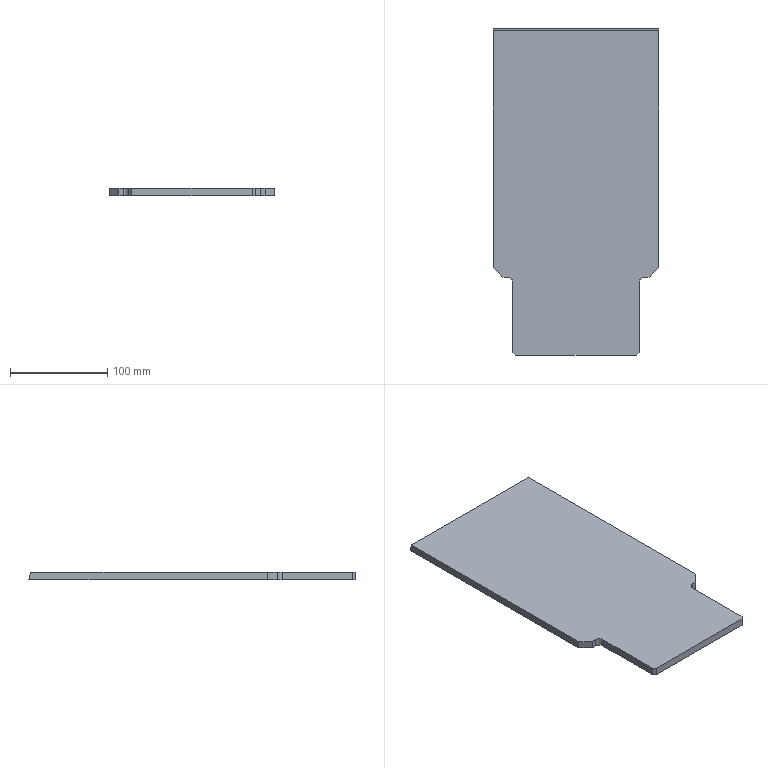Part | STEP file | 001-003-Feeding plate | 1 solid | 16 faces | box 170 x 335 x 8 mm | volume 427857 mm3 | plane 14 | cylinder 2 | commonest cylinder face diameters 10 x2
STEP:
#1=CARTESIAN_POINT('',(0.,0.,0.));
#2=DIRECTION('',(0.,0.,1.));
#3=DIRECTION('',(1.,0.,0.));
#4=AXIS2_PLACEMENT_3D('',#1,#2,#3);
#5=CARTESIAN_POINT('',(85.,-77.5,0.));
#6=VERTEX_POINT('',#5);
#7=CARTESIAN_POINT('',(85.,167.5,0.));
#8=VERTEX_POINT('',#7);
#9=CARTESIAN_POINT('',(85.,167.5,0.));
#10=DIRECTION('',(0.,1.,0.));
#11=VECTOR('',#10,1.);
#12=LINE('',#9,#11);
#13=CARTESIAN_POINT('',(85.,167.5,8.));
#14=DIRECTION('',(-1.,0.,0.));
#15=DIRECTION('',(0.,-1.,0.));
#16=AXIS2_PLACEMENT_3D('',#13,#14,#15);
#17=PLANE('',#16);
#18=CARTESIAN_POINT('',(0.,-8.));
#19=DIRECTION('',(-1.,0.));
#20=VECTOR('',#19,1.);
#21=LINE('',#18,#20);
#22=(GEOMETRIC_REPRESENTATION_CONTEXT(2)PARAMETRIC_REPRESENTATION_CONTEXT()REPRESENTATION_CONTEXT('',''));
#23=DEFINITIONAL_REPRESENTATION('',(#21),#22);
#24=PCURVE('',#17,#23);
#25=CARTESIAN_POINT('',(0.,0.,0.));
#26=DIRECTION('',(0.,0.,1.));
#27=DIRECTION('',(1.,0.,0.));
#28=AXIS2_PLACEMENT_3D('',#25,#26,#27);
#29=PLANE('',#28);
#30=CARTESIAN_POINT('',(85.,167.5));
#31=DIRECTION('',(0.,1.));
#32=VECTOR('',#31,1.);
#33=LINE('',#30,#32);
#34=(GEOMETRIC_REPRESENTATION_CONTEXT(2)PARAMETRIC_REPRESENTATION_CONTEXT()REPRESENTATION_CONTEXT('',''));
#35=DEFINITIONAL_REPRESENTATION('',(#33),#34);
#36=PCURVE('',#29,#35);
#37=SURFACE_CURVE('',#12,(#24,#36),.PCURVE_S1.);
#38=EDGE_CURVE('',#6,#8,#37,.T.);
#39=ORIENTED_EDGE('',*,*,#38,.T.);
#40=CARTESIAN_POINT('',(85.,165.505,8.));
#41=VERTEX_POINT('',#40);
#42=CARTESIAN_POINT('',(85.,167.5,0.));
#43=DIRECTION('',(0.,0.2419,-0.9703));
#44=VECTOR('',#43,1.);
#45=LINE('',#42,#44);
#46=CARTESIAN_POINT('',(0.,-8.));
#47=DIRECTION('',(-0.2419,-0.9703));
#48=VECTOR('',#47,1.);
#49=LINE('',#46,#48);
#50=(GEOMETRIC_REPRESENTATION_CONTEXT(2)PARAMETRIC_REPRESENTATION_CONTEXT()REPRESENTATION_CONTEXT('',''));
#51=DEFINITIONAL_REPRESENTATION('',(#49),#50);
#52=PCURVE('',#17,#51);
#53=CARTESIAN_POINT('',(-85.,167.5,0.));
#54=DIRECTION('',(0.,-0.9703,-0.2419));
#55=DIRECTION('',(0.,0.2419,-0.9703));
#56=AXIS2_PLACEMENT_3D('',#53,#54,#55);
#57=PLANE('',#56);
#58=CARTESIAN_POINT('',(0.,170.));
#59=DIRECTION('',(1.,0.));
#60=VECTOR('',#59,1.);
#61=LINE('',#58,#60);
#62=(GEOMETRIC_REPRESENTATION_CONTEXT(2)PARAMETRIC_REPRESENTATION_CONTEXT()REPRESENTATION_CONTEXT('',''));
#63=DEFINITIONAL_REPRESENTATION('',(#61),#62);
#64=PCURVE('',#57,#63);
#65=SURFACE_CURVE('',#45,(#52,#64),.PCURVE_S1.);
#66=EDGE_CURVE('',#41,#8,#65,.T.);
#67=ORIENTED_EDGE('',*,*,#66,.F.);
#68=CARTESIAN_POINT('',(85.,-77.5,8.));
#69=VERTEX_POINT('',#68);
#70=CARTESIAN_POINT('',(85.,167.5,8.));
#71=DIRECTION('',(0.,1.,0.));
#72=VECTOR('',#71,1.);
#73=LINE('',#70,#72);
#74=CARTESIAN_POINT('',(0.,0.));
#75=DIRECTION('',(-1.,0.));
#76=VECTOR('',#75,1.);
#77=LINE('',#74,#76);
#78=(GEOMETRIC_REPRESENTATION_CONTEXT(2)PARAMETRIC_REPRESENTATION_CONTEXT()REPRESENTATION_CONTEXT('',''));
#79=DEFINITIONAL_REPRESENTATION('',(#77),#78);
#80=PCURVE('',#17,#79);
#81=CARTESIAN_POINT('',(0.,0.,8.));
#82=DIRECTION('',(0.,0.,1.));
#83=DIRECTION('',(1.,0.,0.));
#84=AXIS2_PLACEMENT_3D('',#81,#82,#83);
#85=PLANE('',#84);
#86=CARTESIAN_POINT('',(85.,167.5));
#87=DIRECTION('',(0.,1.));
#88=VECTOR('',#87,1.);
#89=LINE('',#86,#88);
#90=(GEOMETRIC_REPRESENTATION_CONTEXT(2)PARAMETRIC_REPRESENTATION_CONTEXT()REPRESENTATION_CONTEXT('',''));
#91=DEFINITIONAL_REPRESENTATION('',(#89),#90);
#92=PCURVE('',#85,#91);
#93=SURFACE_CURVE('',#73,(#80,#92),.PCURVE_S1.);
#94=EDGE_CURVE('',#69,#41,#93,.T.);
#95=ORIENTED_EDGE('',*,*,#94,.F.);
#96=CARTESIAN_POINT('',(85.,-77.5,0.));
#97=DIRECTION('',(0.,0.,-1.));
#98=VECTOR('',#97,1.);
#99=LINE('',#96,#98);
#100=CARTESIAN_POINT('',(245.,-8.));
#101=DIRECTION('',(0.,-1.));
#102=VECTOR('',#101,1.);
#103=LINE('',#100,#102);
#104=(GEOMETRIC_REPRESENTATION_CONTEXT(2)PARAMETRIC_REPRESENTATION_CONTEXT()REPRESENTATION_CONTEXT('',''));
#105=DEFINITIONAL_REPRESENTATION('',(#103),#104);
#106=PCURVE('',#17,#105);
#107=CARTESIAN_POINT('',(85.,-77.5,8.));
#108=DIRECTION('',(0.7071,-0.7071,0.));
#109=DIRECTION('',(0.,0.,1.));
#110=AXIS2_PLACEMENT_3D('',#107,#108,#109);
#111=PLANE('',#110);
#112=CARTESIAN_POINT('',(-8.,0.));
#113=DIRECTION('',(-1.,0.));
#114=VECTOR('',#113,1.);
#115=LINE('',#112,#114);
#116=(GEOMETRIC_REPRESENTATION_CONTEXT(2)PARAMETRIC_REPRESENTATION_CONTEXT()REPRESENTATION_CONTEXT('',''));
#117=DEFINITIONAL_REPRESENTATION('',(#115),#116);
#118=PCURVE('',#111,#117);
#119=SURFACE_CURVE('',#99,(#106,#118),.PCURVE_S1.);
#120=EDGE_CURVE('',#69,#6,#119,.T.);
#121=ORIENTED_EDGE('',*,*,#120,.T.);
#122=EDGE_LOOP('',(#39,#67,#95,#121));
#123=FACE_BOUND('',#122,.T.);
#124=ADVANCED_FACE('',(#123),#17,.F.);
#125=CARTESIAN_POINT('',(-85.,165.505,8.));
#126=VERTEX_POINT('',#125);
#127=CARTESIAN_POINT('',(-85.,-77.5,8.));
#128=VERTEX_POINT('',#127);
#129=CARTESIAN_POINT('',(-85.,167.5,8.));
#130=DIRECTION('',(0.,-1.,0.));
#131=VECTOR('',#130,1.);
#132=LINE('',#129,#131);
#133=CARTESIAN_POINT('',(-85.,167.5,8.));
#134=DIRECTION('',(1.,0.,0.));
#135=DIRECTION('',(0.,1.,0.));
#136=AXIS2_PLACEMENT_3D('',#133,#134,#135);
#137=PLANE('',#136);
#138=CARTESIAN_POINT('',(0.,0.));
#139=DIRECTION('',(-1.,0.));
#140=VECTOR('',#139,1.);
#141=LINE('',#138,#140);
#142=(GEOMETRIC_REPRESENTATION_CONTEXT(2)PARAMETRIC_REPRESENTATION_CONTEXT()REPRESENTATION_CONTEXT('',''));
#143=DEFINITIONAL_REPRESENTATION('',(#141),#142);
#144=PCURVE('',#137,#143);
#145=CARTESIAN_POINT('',(-85.,167.5));
#146=DIRECTION('',(0.,-1.));
#147=VECTOR('',#146,1.);
#148=LINE('',#145,#147);
#149=(GEOMETRIC_REPRESENTATION_CONTEXT(2)PARAMETRIC_REPRESENTATION_CONTEXT()REPRESENTATION_CONTEXT('',''));
#150=DEFINITIONAL_REPRESENTATION('',(#148),#149);
#151=PCURVE('',#85,#150);
#152=SURFACE_CURVE('',#132,(#144,#151),.PCURVE_S1.);
#153=EDGE_CURVE('',#126,#128,#152,.T.);
#154=ORIENTED_EDGE('',*,*,#153,.F.);
#155=CARTESIAN_POINT('',(-85.,167.5,0.));
#156=VERTEX_POINT('',#155);
#157=CARTESIAN_POINT('',(-85.,167.5,0.));
#158=DIRECTION('',(0.,0.2419,-0.9703));
#159=VECTOR('',#158,1.);
#160=LINE('',#157,#159);
#161=CARTESIAN_POINT('',(0.,-8.));
#162=DIRECTION('',(0.2419,-0.9703));
#163=VECTOR('',#162,1.);
#164=LINE('',#161,#163);
#165=(GEOMETRIC_REPRESENTATION_CONTEXT(2)PARAMETRIC_REPRESENTATION_CONTEXT()REPRESENTATION_CONTEXT('',''));
#166=DEFINITIONAL_REPRESENTATION('',(#164),#165);
#167=PCURVE('',#137,#166);
#168=CARTESIAN_POINT('',(0.,0.));
#169=DIRECTION('',(1.,0.));
#170=VECTOR('',#169,1.);
#171=LINE('',#168,#170);
#172=(GEOMETRIC_REPRESENTATION_CONTEXT(2)PARAMETRIC_REPRESENTATION_CONTEXT()REPRESENTATION_CONTEXT('',''));
#173=DEFINITIONAL_REPRESENTATION('',(#171),#172);
#174=PCURVE('',#57,#173);
#175=SURFACE_CURVE('',#160,(#167,#174),.PCURVE_S1.);
#176=EDGE_CURVE('',#126,#156,#175,.T.);
#177=ORIENTED_EDGE('',*,*,#176,.T.);
#178=CARTESIAN_POINT('',(-85.,-77.5,0.));
#179=VERTEX_POINT('',#178);
#180=CARTESIAN_POINT('',(-85.,167.5,0.));
#181=DIRECTION('',(0.,-1.,0.));
#182=VECTOR('',#181,1.);
#183=LINE('',#180,#182);
#184=CARTESIAN_POINT('',(0.,-8.));
#185=DIRECTION('',(-1.,0.));
#186=VECTOR('',#185,1.);
#187=LINE('',#184,#186);
#188=(GEOMETRIC_REPRESENTATION_CONTEXT(2)PARAMETRIC_REPRESENTATION_CONTEXT()REPRESENTATION_CONTEXT('',''));
#189=DEFINITIONAL_REPRESENTATION('',(#187),#188);
#190=PCURVE('',#137,#189);
#191=CARTESIAN_POINT('',(-85.,167.5));
#192=DIRECTION('',(0.,-1.));
#193=VECTOR('',#192,1.);
#194=LINE('',#191,#193);
#195=(GEOMETRIC_REPRESENTATION_CONTEXT(2)PARAMETRIC_REPRESENTATION_CONTEXT()REPRESENTATION_CONTEXT('',''));
#196=DEFINITIONAL_REPRESENTATION('',(#194),#195);
#197=PCURVE('',#29,#196);
#198=SURFACE_CURVE('',#183,(#190,#197),.PCURVE_S1.);
#199=EDGE_CURVE('',#156,#179,#198,.T.);
#200=ORIENTED_EDGE('',*,*,#199,.T.);
#201=CARTESIAN_POINT('',(-85.,-77.5,8.));
#202=DIRECTION('',(0.,0.,1.));
#203=VECTOR('',#202,1.);
#204=LINE('',#201,#203);
#205=CARTESIAN_POINT('',(-245.,0.));
#206=DIRECTION('',(0.,1.));
#207=VECTOR('',#206,1.);
#208=LINE('',#205,#207);
#209=(GEOMETRIC_REPRESENTATION_CONTEXT(2)PARAMETRIC_REPRESENTATION_CONTEXT()REPRESENTATION_CONTEXT('',''));
#210=DEFINITIONAL_REPRESENTATION('',(#208),#209);
#211=PCURVE('',#137,#210);
#212=CARTESIAN_POINT('',(-75.,-87.5,8.));
#213=DIRECTION('',(-0.7071,-0.7071,0.));
#214=DIRECTION('',(0.,0.,1.));
#215=AXIS2_PLACEMENT_3D('',#212,#213,#214);
#216=PLANE('',#215);
#217=CARTESIAN_POINT('',(0.,14.142));
#218=DIRECTION('',(1.,0.));
#219=VECTOR('',#218,1.);
#220=LINE('',#217,#219);
#221=(GEOMETRIC_REPRESENTATION_CONTEXT(2)PARAMETRIC_REPRESENTATION_CONTEXT()REPRESENTATION_CONTEXT('',''));
#222=DEFINITIONAL_REPRESENTATION('',(#220),#221);
#223=PCURVE('',#216,#222);
#224=SURFACE_CURVE('',#204,(#211,#223),.PCURVE_S1.);
#225=EDGE_CURVE('',#179,#128,#224,.T.);
#226=ORIENTED_EDGE('',*,*,#225,.T.);
#227=EDGE_LOOP('',(#154,#177,#200,#226));
#228=FACE_BOUND('',#227,.T.);
#229=ADVANCED_FACE('',(#228),#137,.F.);
#230=CARTESIAN_POINT('',(-62.,-167.5,8.));
#231=VERTEX_POINT('',#230);
#232=CARTESIAN_POINT('',(62.,-167.5,8.));
#233=VERTEX_POINT('',#232);
#234=CARTESIAN_POINT('',(-85.,-167.5,8.));
#235=DIRECTION('',(1.,0.,0.));
#236=VECTOR('',#235,1.);
#237=LINE('',#234,#236);
#238=CARTESIAN_POINT('',(-85.,-167.5,8.));
#239=DIRECTION('',(0.,1.,0.));
#240=DIRECTION('',(0.,0.,1.));
#241=AXIS2_PLACEMENT_3D('',#238,#239,#240);
#242=PLANE('',#241);
#243=CARTESIAN_POINT('',(0.,0.));
#244=DIRECTION('',(0.,1.));
#245=VECTOR('',#244,1.);
#246=LINE('',#243,#245);
#247=(GEOMETRIC_REPRESENTATION_CONTEXT(2)PARAMETRIC_REPRESENTATION_CONTEXT()REPRESENTATION_CONTEXT('',''));
#248=DEFINITIONAL_REPRESENTATION('',(#246),#247);
#249=PCURVE('',#242,#248);
#250=CARTESIAN_POINT('',(-85.,-167.5));
#251=DIRECTION('',(1.,0.));
#252=VECTOR('',#251,1.);
#253=LINE('',#250,#252);
#254=(GEOMETRIC_REPRESENTATION_CONTEXT(2)PARAMETRIC_REPRESENTATION_CONTEXT()REPRESENTATION_CONTEXT('',''));
#255=DEFINITIONAL_REPRESENTATION('',(#253),#254);
#256=PCURVE('',#85,#255);
#257=SURFACE_CURVE('',#237,(#249,#256),.PCURVE_S1.);
#258=EDGE_CURVE('',#231,#233,#257,.T.);
#259=ORIENTED_EDGE('',*,*,#258,.F.);
#260=CARTESIAN_POINT('',(-62.,-167.5,0.));
#261=VERTEX_POINT('',#260);
#262=CARTESIAN_POINT('',(-62.,-167.5,0.));
#263=DIRECTION('',(0.,0.,-1.));
#264=VECTOR('',#263,1.);
#265=LINE('',#262,#264);
#266=CARTESIAN_POINT('',(-8.,23.));
#267=DIRECTION('',(-1.,0.));
#268=VECTOR('',#267,1.);
#269=LINE('',#266,#268);
#270=(GEOMETRIC_REPRESENTATION_CONTEXT(2)PARAMETRIC_REPRESENTATION_CONTEXT()REPRESENTATION_CONTEXT('',''));
#271=DEFINITIONAL_REPRESENTATION('',(#269),#270);
#272=PCURVE('',#242,#271);
#273=CARTESIAN_POINT('',(-62.,-167.5,8.));
#274=DIRECTION('',(-0.7071,-0.7071,0.));
#275=DIRECTION('',(0.,0.,1.));
#276=AXIS2_PLACEMENT_3D('',#273,#274,#275);
#277=PLANE('',#276);
#278=CARTESIAN_POINT('',(-8.,0.));
#279=DIRECTION('',(-1.,0.));
#280=VECTOR('',#279,1.);
#281=LINE('',#278,#280);
#282=(GEOMETRIC_REPRESENTATION_CONTEXT(2)PARAMETRIC_REPRESENTATION_CONTEXT()REPRESENTATION_CONTEXT('',''));
#283=DEFINITIONAL_REPRESENTATION('',(#281),#282);
#284=PCURVE('',#277,#283);
#285=SURFACE_CURVE('',#265,(#272,#284),.PCURVE_S1.);
#286=EDGE_CURVE('',#231,#261,#285,.T.);
#287=ORIENTED_EDGE('',*,*,#286,.T.);
#288=CARTESIAN_POINT('',(62.,-167.5,0.));
#289=VERTEX_POINT('',#288);
#290=CARTESIAN_POINT('',(-85.,-167.5,0.));
#291=DIRECTION('',(1.,0.,0.));
#292=VECTOR('',#291,1.);
#293=LINE('',#290,#292);
#294=CARTESIAN_POINT('',(-8.,0.));
#295=DIRECTION('',(0.,1.));
#296=VECTOR('',#295,1.);
#297=LINE('',#294,#296);
#298=(GEOMETRIC_REPRESENTATION_CONTEXT(2)PARAMETRIC_REPRESENTATION_CONTEXT()REPRESENTATION_CONTEXT('',''));
#299=DEFINITIONAL_REPRESENTATION('',(#297),#298);
#300=PCURVE('',#242,#299);
#301=CARTESIAN_POINT('',(-85.,-167.5));
#302=DIRECTION('',(1.,0.));
#303=VECTOR('',#302,1.);
#304=LINE('',#301,#303);
#305=(GEOMETRIC_REPRESENTATION_CONTEXT(2)PARAMETRIC_REPRESENTATION_CONTEXT()REPRESENTATION_CONTEXT('',''));
#306=DEFINITIONAL_REPRESENTATION('',(#304),#305);
#307=PCURVE('',#29,#306);
#308=SURFACE_CURVE('',#293,(#300,#307),.PCURVE_S1.);
#309=EDGE_CURVE('',#261,#289,#308,.T.);
#310=ORIENTED_EDGE('',*,*,#309,.T.);
#311=CARTESIAN_POINT('',(62.,-167.5,8.));
#312=DIRECTION('',(0.,0.,1.));
#313=VECTOR('',#312,1.);
#314=LINE('',#311,#313);
#315=CARTESIAN_POINT('',(0.,147.));
#316=DIRECTION('',(1.,0.));
#317=VECTOR('',#316,1.);
#318=LINE('',#315,#317);
#319=(GEOMETRIC_REPRESENTATION_CONTEXT(2)PARAMETRIC_REPRESENTATION_CONTEXT()REPRESENTATION_CONTEXT('',''));
#320=DEFINITIONAL_REPRESENTATION('',(#318),#319);
#321=PCURVE('',#242,#320);
#322=CARTESIAN_POINT('',(65.,-164.5,8.));
#323=DIRECTION('',(0.7071,-0.7071,0.));
#324=DIRECTION('',(0.,0.,1.));
#325=AXIS2_PLACEMENT_3D('',#322,#323,#324);
#326=PLANE('',#325);
#327=CARTESIAN_POINT('',(0.,4.243));
#328=DIRECTION('',(1.,0.));
#329=VECTOR('',#328,1.);
#330=LINE('',#327,#329);
#331=(GEOMETRIC_REPRESENTATION_CONTEXT(2)PARAMETRIC_REPRESENTATION_CONTEXT()REPRESENTATION_CONTEXT('',''));
#332=DEFINITIONAL_REPRESENTATION('',(#330),#331);
#333=PCURVE('',#326,#332);
#334=SURFACE_CURVE('',#314,(#321,#333),.PCURVE_S1.);
#335=EDGE_CURVE('',#289,#233,#334,.T.);
#336=ORIENTED_EDGE('',*,*,#335,.T.);
#337=EDGE_LOOP('',(#259,#287,#310,#336));
#338=FACE_BOUND('',#337,.T.);
#339=ADVANCED_FACE('',(#338),#242,.F.);
#340=CARTESIAN_POINT('',(-85.,165.505,8.));
#341=DIRECTION('',(1.,0.,0.));
#342=VECTOR('',#341,1.);
#343=LINE('',#340,#342);
#344=CARTESIAN_POINT('',(-85.,165.505));
#345=DIRECTION('',(1.,0.));
#346=VECTOR('',#345,1.);
#347=LINE('',#344,#346);
#348=(GEOMETRIC_REPRESENTATION_CONTEXT(2)PARAMETRIC_REPRESENTATION_CONTEXT()REPRESENTATION_CONTEXT('',''));
#349=DEFINITIONAL_REPRESENTATION('',(#347),#348);
#350=PCURVE('',#85,#349);
#351=CARTESIAN_POINT('',(-8.245,0.));
#352=DIRECTION('',(0.,1.));
#353=VECTOR('',#352,1.);
#354=LINE('',#351,#353);
#355=(GEOMETRIC_REPRESENTATION_CONTEXT(2)PARAMETRIC_REPRESENTATION_CONTEXT()REPRESENTATION_CONTEXT('',''));
#356=DEFINITIONAL_REPRESENTATION('',(#354),#355);
#357=PCURVE('',#57,#356);
#358=SURFACE_CURVE('',#343,(#350,#357),.PCURVE_S1.);
#359=EDGE_CURVE('',#126,#41,#358,.T.);
#360=ORIENTED_EDGE('',*,*,#359,.F.);
#361=ORIENTED_EDGE('',*,*,#153,.T.);
#362=CARTESIAN_POINT('',(-75.,-87.5,8.));
#363=VERTEX_POINT('',#362);
#364=CARTESIAN_POINT('',(-81.25,-81.25,8.));
#365=DIRECTION('',(0.7071,-0.7071,0.));
#366=VECTOR('',#365,1.);
#367=LINE('',#364,#366);
#368=CARTESIAN_POINT('',(-81.25,-81.25));
#369=DIRECTION('',(0.7071,-0.7071));
#370=VECTOR('',#369,1.);
#371=LINE('',#368,#370);
#372=(GEOMETRIC_REPRESENTATION_CONTEXT(2)PARAMETRIC_REPRESENTATION_CONTEXT()REPRESENTATION_CONTEXT('',''));
#373=DEFINITIONAL_REPRESENTATION('',(#371),#372);
#374=PCURVE('',#85,#373);
#375=CARTESIAN_POINT('',(0.,8.839));
#376=DIRECTION('',(0.,-1.));
#377=VECTOR('',#376,1.);
#378=LINE('',#375,#377);
#379=(GEOMETRIC_REPRESENTATION_CONTEXT(2)PARAMETRIC_REPRESENTATION_CONTEXT()REPRESENTATION_CONTEXT('',''));
#380=DEFINITIONAL_REPRESENTATION('',(#378),#379);
#381=PCURVE('',#216,#380);
#382=SURFACE_CURVE('',#367,(#374,#381),.PCURVE_S1.);
#383=EDGE_CURVE('',#128,#363,#382,.T.);
#384=ORIENTED_EDGE('',*,*,#383,.T.);
#385=CARTESIAN_POINT('',(-70.,-87.5,8.));
#386=VERTEX_POINT('',#385);
#387=CARTESIAN_POINT('',(-85.,-87.5,8.));
#388=DIRECTION('',(-1.,0.,0.));
#389=VECTOR('',#388,1.);
#390=LINE('',#387,#389);
#391=CARTESIAN_POINT('',(-85.,-87.5));
#392=DIRECTION('',(-1.,0.));
#393=VECTOR('',#392,1.);
#394=LINE('',#391,#393);
#395=(GEOMETRIC_REPRESENTATION_CONTEXT(2)PARAMETRIC_REPRESENTATION_CONTEXT()REPRESENTATION_CONTEXT('',''));
#396=DEFINITIONAL_REPRESENTATION('',(#394),#395);
#397=PCURVE('',#85,#396);
#398=CARTESIAN_POINT('',(-85.,-87.5,8.));
#399=DIRECTION('',(0.,-1.,0.));
#400=DIRECTION('',(0.,0.,-1.));
#401=AXIS2_PLACEMENT_3D('',#398,#399,#400);
#402=PLANE('',#401);
#403=CARTESIAN_POINT('',(0.,0.));
#404=DIRECTION('',(0.,-1.));
#405=VECTOR('',#404,1.);
#406=LINE('',#403,#405);
#407=(GEOMETRIC_REPRESENTATION_CONTEXT(2)PARAMETRIC_REPRESENTATION_CONTEXT()REPRESENTATION_CONTEXT('',''));
#408=DEFINITIONAL_REPRESENTATION('',(#406),#407);
#409=PCURVE('',#402,#408);
#410=SURFACE_CURVE('',#390,(#397,#409),.PCURVE_S1.);
#411=EDGE_CURVE('',#386,#363,#410,.T.);
#412=ORIENTED_EDGE('',*,*,#411,.F.);
#413=CARTESIAN_POINT('',(-65.,-92.5,8.));
#414=VERTEX_POINT('',#413);
#415=CARTESIAN_POINT('',(-70.,-92.5,8.));
#416=DIRECTION('',(0.,0.,-1.));
#417=DIRECTION('',(1.,0.,0.));
#418=AXIS2_PLACEMENT_3D('',#415,#416,#417);
#419=CIRCLE('',#418,5.);
#420=CARTESIAN_POINT('',(-65.,-92.5));
#421=CARTESIAN_POINT('',(-65.,-101.16));
#422=CARTESIAN_POINT('',(-72.5,-96.83));
#423=CARTESIAN_POINT('',(-80.,-92.5));
#424=CARTESIAN_POINT('',(-72.5,-88.17));
#425=CARTESIAN_POINT('',(-65.,-83.84));
#426=CARTESIAN_POINT('',(-65.,-92.5));
#427=(BOUNDED_CURVE()B_SPLINE_CURVE(2,(#420,#421,#422,#423,#424,#425,#426),.UNSPECIFIED.,.T.,.F.)B_SPLINE_CURVE_WITH_KNOTS((1,2,2,2,2,1),(-2.094,0.,2.094,4.189,6.283,8.378),.UNSPECIFIED.)CURVE()GEOMETRIC_REPRESENTATION_ITEM()RATIONAL_B_SPLINE_CURVE((1.,0.5,1.,0.5,1.,0.5,1.))REPRESENTATION_ITEM(''));
#428=(GEOMETRIC_REPRESENTATION_CONTEXT(2)PARAMETRIC_REPRESENTATION_CONTEXT()REPRESENTATION_CONTEXT('',''));
#429=DEFINITIONAL_REPRESENTATION('',(#427),#428);
#430=PCURVE('',#85,#429);
#431=CARTESIAN_POINT('',(-70.,-92.5,8.));
#432=DIRECTION('',(0.,0.,1.));
#433=DIRECTION('',(1.,0.,0.));
#434=AXIS2_PLACEMENT_3D('',#431,#432,#433);
#435=CYLINDRICAL_SURFACE('',#434,5.);
#436=CARTESIAN_POINT('',(6.283,0.));
#437=DIRECTION('',(-1.,0.));
#438=VECTOR('',#437,1.);
#439=LINE('',#436,#438);
#440=(GEOMETRIC_REPRESENTATION_CONTEXT(2)PARAMETRIC_REPRESENTATION_CONTEXT()REPRESENTATION_CONTEXT('',''));
#441=DEFINITIONAL_REPRESENTATION('',(#439),#440);
#442=PCURVE('',#435,#441);
#443=SURFACE_CURVE('',#419,(#430,#442),.PCURVE_S1.);
#444=EDGE_CURVE('',#386,#414,#443,.T.);
#445=ORIENTED_EDGE('',*,*,#444,.T.);
#446=CARTESIAN_POINT('',(-65.,-164.5,8.));
#447=VERTEX_POINT('',#446);
#448=CARTESIAN_POINT('',(-65.,-167.5,8.));
#449=DIRECTION('',(0.,1.,0.));
#450=VECTOR('',#449,1.);
#451=LINE('',#448,#450);
#452=CARTESIAN_POINT('',(-65.,-167.5));
#453=DIRECTION('',(0.,1.));
#454=VECTOR('',#453,1.);
#455=LINE('',#452,#454);
#456=(GEOMETRIC_REPRESENTATION_CONTEXT(2)PARAMETRIC_REPRESENTATION_CONTEXT()REPRESENTATION_CONTEXT('',''));
#457=DEFINITIONAL_REPRESENTATION('',(#455),#456);
#458=PCURVE('',#85,#457);
#459=CARTESIAN_POINT('',(-65.,-167.5,8.));
#460=DIRECTION('',(-1.,0.,0.));
#461=DIRECTION('',(0.,-1.,0.));
#462=AXIS2_PLACEMENT_3D('',#459,#460,#461);
#463=PLANE('',#462);
#464=CARTESIAN_POINT('',(0.,0.));
#465=DIRECTION('',(-1.,0.));
#466=VECTOR('',#465,1.);
#467=LINE('',#464,#466);
#468=(GEOMETRIC_REPRESENTATION_CONTEXT(2)PARAMETRIC_REPRESENTATION_CONTEXT()REPRESENTATION_CONTEXT('',''));
#469=DEFINITIONAL_REPRESENTATION('',(#467),#468);
#470=PCURVE('',#463,#469);
#471=SURFACE_CURVE('',#451,(#458,#470),.PCURVE_S1.);
#472=EDGE_CURVE('',#447,#414,#471,.T.);
#473=ORIENTED_EDGE('',*,*,#472,.F.);
#474=CARTESIAN_POINT('',(-114.75,-114.75,8.));
#475=DIRECTION('',(0.7071,-0.7071,0.));
#476=VECTOR('',#475,1.);
#477=LINE('',#474,#476);
#478=CARTESIAN_POINT('',(-114.75,-114.75));
#479=DIRECTION('',(0.7071,-0.7071));
#480=VECTOR('',#479,1.);
#481=LINE('',#478,#480);
#482=(GEOMETRIC_REPRESENTATION_CONTEXT(2)PARAMETRIC_REPRESENTATION_CONTEXT()REPRESENTATION_CONTEXT('',''));
#483=DEFINITIONAL_REPRESENTATION('',(#481),#482);
#484=PCURVE('',#85,#483);
#485=CARTESIAN_POINT('',(0.,74.6));
#486=DIRECTION('',(0.,-1.));
#487=VECTOR('',#486,1.);
#488=LINE('',#485,#487);
#489=(GEOMETRIC_REPRESENTATION_CONTEXT(2)PARAMETRIC_REPRESENTATION_CONTEXT()REPRESENTATION_CONTEXT('',''));
#490=DEFINITIONAL_REPRESENTATION('',(#488),#489);
#491=PCURVE('',#277,#490);
#492=SURFACE_CURVE('',#477,(#484,#491),.PCURVE_S1.);
#493=EDGE_CURVE('',#447,#231,#492,.T.);
#494=ORIENTED_EDGE('',*,*,#493,.T.);
#495=ORIENTED_EDGE('',*,*,#258,.T.);
#496=CARTESIAN_POINT('',(65.,-164.5,8.));
#497=VERTEX_POINT('',#496);
#498=CARTESIAN_POINT('',(114.75,-114.75,8.));
#499=DIRECTION('',(0.7071,0.7071,0.));
#500=VECTOR('',#499,1.);
#501=LINE('',#498,#500);
#502=CARTESIAN_POINT('',(114.75,-114.75));
#503=DIRECTION('',(0.7071,0.7071));
#504=VECTOR('',#503,1.);
#505=LINE('',#502,#504);
#506=(GEOMETRIC_REPRESENTATION_CONTEXT(2)PARAMETRIC_REPRESENTATION_CONTEXT()REPRESENTATION_CONTEXT('',''));
#507=DEFINITIONAL_REPRESENTATION('',(#505),#506);
#508=PCURVE('',#85,#507);
#509=CARTESIAN_POINT('',(0.,-70.357));
#510=DIRECTION('',(0.,-1.));
#511=VECTOR('',#510,1.);
#512=LINE('',#509,#511);
#513=(GEOMETRIC_REPRESENTATION_CONTEXT(2)PARAMETRIC_REPRESENTATION_CONTEXT()REPRESENTATION_CONTEXT('',''));
#514=DEFINITIONAL_REPRESENTATION('',(#512),#513);
#515=PCURVE('',#326,#514);
#516=SURFACE_CURVE('',#501,(#508,#515),.PCURVE_S1.);
#517=EDGE_CURVE('',#233,#497,#516,.T.);
#518=ORIENTED_EDGE('',*,*,#517,.T.);
#519=CARTESIAN_POINT('',(65.,-92.5,8.));
#520=VERTEX_POINT('',#519);
#521=CARTESIAN_POINT('',(65.,-167.5,8.));
#522=DIRECTION('',(0.,-1.,0.));
#523=VECTOR('',#522,1.);
#524=LINE('',#521,#523);
#525=CARTESIAN_POINT('',(65.,-167.5));
#526=DIRECTION('',(0.,-1.));
#527=VECTOR('',#526,1.);
#528=LINE('',#525,#527);
#529=(GEOMETRIC_REPRESENTATION_CONTEXT(2)PARAMETRIC_REPRESENTATION_CONTEXT()REPRESENTATION_CONTEXT('',''));
#530=DEFINITIONAL_REPRESENTATION('',(#528),#529);
#531=PCURVE('',#85,#530);
#532=CARTESIAN_POINT('',(65.,-167.5,8.));
#533=DIRECTION('',(1.,0.,0.));
#534=DIRECTION('',(0.,1.,0.));
#535=AXIS2_PLACEMENT_3D('',#532,#533,#534);
#536=PLANE('',#535);
#537=CARTESIAN_POINT('',(0.,0.));
#538=DIRECTION('',(-1.,0.));
#539=VECTOR('',#538,1.);
#540=LINE('',#537,#539);
#541=(GEOMETRIC_REPRESENTATION_CONTEXT(2)PARAMETRIC_REPRESENTATION_CONTEXT()REPRESENTATION_CONTEXT('',''));
#542=DEFINITIONAL_REPRESENTATION('',(#540),#541);
#543=PCURVE('',#536,#542);
#544=SURFACE_CURVE('',#524,(#531,#543),.PCURVE_S1.);
#545=EDGE_CURVE('',#520,#497,#544,.T.);
#546=ORIENTED_EDGE('',*,*,#545,.F.);
#547=CARTESIAN_POINT('',(70.,-87.5,8.));
#548=VERTEX_POINT('',#547);
#549=CARTESIAN_POINT('',(70.,-92.5,8.));
#550=DIRECTION('',(0.,0.,-1.));
#551=DIRECTION('',(1.,0.,0.));
#552=AXIS2_PLACEMENT_3D('',#549,#550,#551);
#553=CIRCLE('',#552,5.);
#554=CARTESIAN_POINT('',(75.,-92.5));
#555=CARTESIAN_POINT('',(75.,-101.16));
#556=CARTESIAN_POINT('',(67.5,-96.83));
#557=CARTESIAN_POINT('',(60.,-92.5));
#558=CARTESIAN_POINT('',(67.5,-88.17));
#559=CARTESIAN_POINT('',(75.,-83.84));
#560=CARTESIAN_POINT('',(75.,-92.5));
#561=(BOUNDED_CURVE()B_SPLINE_CURVE(2,(#554,#555,#556,#557,#558,#559,#560),.UNSPECIFIED.,.T.,.F.)B_SPLINE_CURVE_WITH_KNOTS((1,2,2,2,2,1),(-2.094,0.,2.094,4.189,6.283,8.378),.UNSPECIFIED.)CURVE()GEOMETRIC_REPRESENTATION_ITEM()RATIONAL_B_SPLINE_CURVE((1.,0.5,1.,0.5,1.,0.5,1.))REPRESENTATION_ITEM(''));
#562=(GEOMETRIC_REPRESENTATION_CONTEXT(2)PARAMETRIC_REPRESENTATION_CONTEXT()REPRESENTATION_CONTEXT('',''));
#563=DEFINITIONAL_REPRESENTATION('',(#561),#562);
#564=PCURVE('',#85,#563);
#565=CARTESIAN_POINT('',(70.,-92.5,8.));
#566=DIRECTION('',(0.,0.,1.));
#567=DIRECTION('',(1.,0.,0.));
#568=AXIS2_PLACEMENT_3D('',#565,#566,#567);
#569=CYLINDRICAL_SURFACE('',#568,5.);
#570=CARTESIAN_POINT('',(6.283,0.));
#571=DIRECTION('',(-1.,0.));
#572=VECTOR('',#571,1.);
#573=LINE('',#570,#572);
#574=(GEOMETRIC_REPRESENTATION_CONTEXT(2)PARAMETRIC_REPRESENTATION_CONTEXT()REPRESENTATION_CONTEXT('',''));
#575=DEFINITIONAL_REPRESENTATION('',(#573),#574);
#576=PCURVE('',#569,#575);
#577=SURFACE_CURVE('',#553,(#564,#576),.PCURVE_S1.);
#578=EDGE_CURVE('',#520,#548,#577,.T.);
#579=ORIENTED_EDGE('',*,*,#578,.T.);
#580=CARTESIAN_POINT('',(75.,-87.5,8.));
#581=VERTEX_POINT('',#580);
#582=CARTESIAN_POINT('',(85.,-87.5,8.));
#583=DIRECTION('',(-1.,0.,0.));
#584=VECTOR('',#583,1.);
#585=LINE('',#582,#584);
#586=CARTESIAN_POINT('',(85.,-87.5));
#587=DIRECTION('',(-1.,0.));
#588=VECTOR('',#587,1.);
#589=LINE('',#586,#588);
#590=(GEOMETRIC_REPRESENTATION_CONTEXT(2)PARAMETRIC_REPRESENTATION_CONTEXT()REPRESENTATION_CONTEXT('',''));
#591=DEFINITIONAL_REPRESENTATION('',(#589),#590);
#592=PCURVE('',#85,#591);
#593=CARTESIAN_POINT('',(85.,-87.5,8.));
#594=DIRECTION('',(0.,-1.,0.));
#595=DIRECTION('',(1.,0.,0.));
#596=AXIS2_PLACEMENT_3D('',#593,#594,#595);
#597=PLANE('',#596);
#598=CARTESIAN_POINT('',(0.,0.));
#599=DIRECTION('',(-1.,0.));
#600=VECTOR('',#599,1.);
#601=LINE('',#598,#600);
#602=(GEOMETRIC_REPRESENTATION_CONTEXT(2)PARAMETRIC_REPRESENTATION_CONTEXT()REPRESENTATION_CONTEXT('',''));
#603=DEFINITIONAL_REPRESENTATION('',(#601),#602);
#604=PCURVE('',#597,#603);
#605=SURFACE_CURVE('',#585,(#592,#604),.PCURVE_S1.);
#606=EDGE_CURVE('',#581,#548,#605,.T.);
#607=ORIENTED_EDGE('',*,*,#606,.F.);
#608=CARTESIAN_POINT('',(81.25,-81.25,8.));
#609=DIRECTION('',(0.7071,0.7071,0.));
#610=VECTOR('',#609,1.);
#611=LINE('',#608,#610);
#612=CARTESIAN_POINT('',(81.25,-81.25));
#613=DIRECTION('',(0.7071,0.7071));
#614=VECTOR('',#613,1.);
#615=LINE('',#612,#614);
#616=(GEOMETRIC_REPRESENTATION_CONTEXT(2)PARAMETRIC_REPRESENTATION_CONTEXT()REPRESENTATION_CONTEXT('',''));
#617=DEFINITIONAL_REPRESENTATION('',(#615),#616);
#618=PCURVE('',#85,#617);
#619=CARTESIAN_POINT('',(0.,5.303));
#620=DIRECTION('',(0.,-1.));
#621=VECTOR('',#620,1.);
#622=LINE('',#619,#621);
#623=(GEOMETRIC_REPRESENTATION_CONTEXT(2)PARAMETRIC_REPRESENTATION_CONTEXT()REPRESENTATION_CONTEXT('',''));
#624=DEFINITIONAL_REPRESENTATION('',(#622),#623);
#625=PCURVE('',#111,#624);
#626=SURFACE_CURVE('',#611,(#618,#625),.PCURVE_S1.);
#627=EDGE_CURVE('',#581,#69,#626,.T.);
#628=ORIENTED_EDGE('',*,*,#627,.T.);
#629=ORIENTED_EDGE('',*,*,#94,.T.);
#630=EDGE_LOOP('',(#360,#361,#384,#412,#445,#473,#494,#495,#518,#546,#579,#607,#628,#629));
#631=FACE_BOUND('',#630,.T.);
#632=ADVANCED_FACE('',(#631),#85,.T.);
#633=ORIENTED_EDGE('',*,*,#309,.F.);
#634=CARTESIAN_POINT('',(-65.,-164.5,0.));
#635=VERTEX_POINT('',#634);
#636=CARTESIAN_POINT('',(-62.,-167.5,0.));
#637=DIRECTION('',(-0.7071,0.7071,0.));
#638=VECTOR('',#637,1.);
#639=LINE('',#636,#638);
#640=CARTESIAN_POINT('',(-62.,-167.5));
#641=DIRECTION('',(-0.7071,0.7071));
#642=VECTOR('',#641,1.);
#643=LINE('',#640,#642);
#644=(GEOMETRIC_REPRESENTATION_CONTEXT(2)PARAMETRIC_REPRESENTATION_CONTEXT()REPRESENTATION_CONTEXT('',''));
#645=DEFINITIONAL_REPRESENTATION('',(#643),#644);
#646=PCURVE('',#29,#645);
#647=CARTESIAN_POINT('',(-8.,0.));
#648=DIRECTION('',(0.,1.));
#649=VECTOR('',#648,1.);
#650=LINE('',#647,#649);
#651=(GEOMETRIC_REPRESENTATION_CONTEXT(2)PARAMETRIC_REPRESENTATION_CONTEXT()REPRESENTATION_CONTEXT('',''));
#652=DEFINITIONAL_REPRESENTATION('',(#650),#651);
#653=PCURVE('',#277,#652);
#654=SURFACE_CURVE('',#639,(#646,#653),.PCURVE_S1.);
#655=EDGE_CURVE('',#261,#635,#654,.T.);
#656=ORIENTED_EDGE('',*,*,#655,.T.);
#657=CARTESIAN_POINT('',(-65.,-92.5,0.));
#658=VERTEX_POINT('',#657);
#659=CARTESIAN_POINT('',(-65.,-167.5,0.));
#660=DIRECTION('',(0.,1.,0.));
#661=VECTOR('',#660,1.);
#662=LINE('',#659,#661);
#663=CARTESIAN_POINT('',(-65.,-167.5));
#664=DIRECTION('',(0.,1.));
#665=VECTOR('',#664,1.);
#666=LINE('',#663,#665);
#667=(GEOMETRIC_REPRESENTATION_CONTEXT(2)PARAMETRIC_REPRESENTATION_CONTEXT()REPRESENTATION_CONTEXT('',''));
#668=DEFINITIONAL_REPRESENTATION('',(#666),#667);
#669=PCURVE('',#29,#668);
#670=CARTESIAN_POINT('',(0.,-8.));
#671=DIRECTION('',(-1.,0.));
#672=VECTOR('',#671,1.);
#673=LINE('',#670,#672);
#674=(GEOMETRIC_REPRESENTATION_CONTEXT(2)PARAMETRIC_REPRESENTATION_CONTEXT()REPRESENTATION_CONTEXT('',''));
#675=DEFINITIONAL_REPRESENTATION('',(#673),#674);
#676=PCURVE('',#463,#675);
#677=SURFACE_CURVE('',#662,(#669,#676),.PCURVE_S1.);
#678=EDGE_CURVE('',#635,#658,#677,.T.);
#679=ORIENTED_EDGE('',*,*,#678,.T.);
#680=CARTESIAN_POINT('',(-70.,-87.5,0.));
#681=VERTEX_POINT('',#680);
#682=CARTESIAN_POINT('',(-70.,-92.5,0.));
#683=DIRECTION('',(0.,0.,1.));
#684=DIRECTION('',(1.,0.,0.));
#685=AXIS2_PLACEMENT_3D('',#682,#683,#684);
#686=CIRCLE('',#685,5.);
#687=CARTESIAN_POINT('',(-70.,-92.5));
#688=DIRECTION('',(1.,0.));
#689=AXIS2_PLACEMENT_2D('',#687,#688);
#690=CIRCLE('',#689,5.);
#691=(GEOMETRIC_REPRESENTATION_CONTEXT(2)PARAMETRIC_REPRESENTATION_CONTEXT()REPRESENTATION_CONTEXT('',''));
#692=DEFINITIONAL_REPRESENTATION('',(#690),#691);
#693=PCURVE('',#29,#692);
#694=CARTESIAN_POINT('',(0.,-8.));
#695=DIRECTION('',(1.,0.));
#696=VECTOR('',#695,1.);
#697=LINE('',#694,#696);
#698=(GEOMETRIC_REPRESENTATION_CONTEXT(2)PARAMETRIC_REPRESENTATION_CONTEXT()REPRESENTATION_CONTEXT('',''));
#699=DEFINITIONAL_REPRESENTATION('',(#697),#698);
#700=PCURVE('',#435,#699);
#701=SURFACE_CURVE('',#686,(#693,#700),.PCURVE_S1.);
#702=EDGE_CURVE('',#658,#681,#701,.T.);
#703=ORIENTED_EDGE('',*,*,#702,.T.);
#704=CARTESIAN_POINT('',(-75.,-87.5,0.));
#705=VERTEX_POINT('',#704);
#706=CARTESIAN_POINT('',(-85.,-87.5,0.));
#707=DIRECTION('',(-1.,0.,0.));
#708=VECTOR('',#707,1.);
#709=LINE('',#706,#708);
#710=CARTESIAN_POINT('',(-85.,-87.5));
#711=DIRECTION('',(-1.,0.));
#712=VECTOR('',#711,1.);
#713=LINE('',#710,#712);
#714=(GEOMETRIC_REPRESENTATION_CONTEXT(2)PARAMETRIC_REPRESENTATION_CONTEXT()REPRESENTATION_CONTEXT('',''));
#715=DEFINITIONAL_REPRESENTATION('',(#713),#714);
#716=PCURVE('',#29,#715);
#717=CARTESIAN_POINT('',(8.,0.));
#718=DIRECTION('',(0.,-1.));
#719=VECTOR('',#718,1.);
#720=LINE('',#717,#719);
#721=(GEOMETRIC_REPRESENTATION_CONTEXT(2)PARAMETRIC_REPRESENTATION_CONTEXT()REPRESENTATION_CONTEXT('',''));
#722=DEFINITIONAL_REPRESENTATION('',(#720),#721);
#723=PCURVE('',#402,#722);
#724=SURFACE_CURVE('',#709,(#716,#723),.PCURVE_S1.);
#725=EDGE_CURVE('',#681,#705,#724,.T.);
#726=ORIENTED_EDGE('',*,*,#725,.T.);
#727=CARTESIAN_POINT('',(-75.,-87.5,0.));
#728=DIRECTION('',(-0.7071,0.7071,0.));
#729=VECTOR('',#728,1.);
#730=LINE('',#727,#729);
#731=CARTESIAN_POINT('',(-75.,-87.5));
#732=DIRECTION('',(-0.7071,0.7071));
#733=VECTOR('',#732,1.);
#734=LINE('',#731,#733);
#735=(GEOMETRIC_REPRESENTATION_CONTEXT(2)PARAMETRIC_REPRESENTATION_CONTEXT()REPRESENTATION_CONTEXT('',''));
#736=DEFINITIONAL_REPRESENTATION('',(#734),#735);
#737=PCURVE('',#29,#736);
#738=CARTESIAN_POINT('',(-8.,0.));
#739=DIRECTION('',(0.,1.));
#740=VECTOR('',#739,1.);
#741=LINE('',#738,#740);
#742=(GEOMETRIC_REPRESENTATION_CONTEXT(2)PARAMETRIC_REPRESENTATION_CONTEXT()REPRESENTATION_CONTEXT('',''));
#743=DEFINITIONAL_REPRESENTATION('',(#741),#742);
#744=PCURVE('',#216,#743);
#745=SURFACE_CURVE('',#730,(#737,#744),.PCURVE_S1.);
#746=EDGE_CURVE('',#705,#179,#745,.T.);
#747=ORIENTED_EDGE('',*,*,#746,.T.);
#748=ORIENTED_EDGE('',*,*,#199,.F.);
#749=CARTESIAN_POINT('',(-85.,167.5,0.));
#750=DIRECTION('',(-1.,0.,0.));
#751=VECTOR('',#750,1.);
#752=LINE('',#749,#751);
#753=CARTESIAN_POINT('',(-85.,167.5));
#754=DIRECTION('',(-1.,0.));
#755=VECTOR('',#754,1.);
#756=LINE('',#753,#755);
#757=(GEOMETRIC_REPRESENTATION_CONTEXT(2)PARAMETRIC_REPRESENTATION_CONTEXT()REPRESENTATION_CONTEXT('',''));
#758=DEFINITIONAL_REPRESENTATION('',(#756),#757);
#759=PCURVE('',#29,#758);
#760=CARTESIAN_POINT('',(0.,0.));
#761=DIRECTION('',(0.,-1.));
#762=VECTOR('',#761,1.);
#763=LINE('',#760,#762);
#764=(GEOMETRIC_REPRESENTATION_CONTEXT(2)PARAMETRIC_REPRESENTATION_CONTEXT()REPRESENTATION_CONTEXT('',''));
#765=DEFINITIONAL_REPRESENTATION('',(#763),#764);
#766=PCURVE('',#57,#765);
#767=SURFACE_CURVE('',#752,(#759,#766),.PCURVE_S1.);
#768=EDGE_CURVE('',#8,#156,#767,.T.);
#769=ORIENTED_EDGE('',*,*,#768,.F.);
#770=ORIENTED_EDGE('',*,*,#38,.F.);
#771=CARTESIAN_POINT('',(75.,-87.5,0.));
#772=VERTEX_POINT('',#771);
#773=CARTESIAN_POINT('',(85.,-77.5,0.));
#774=DIRECTION('',(-0.7071,-0.7071,0.));
#775=VECTOR('',#774,1.);
#776=LINE('',#773,#775);
#777=CARTESIAN_POINT('',(85.,-77.5));
#778=DIRECTION('',(-0.7071,-0.7071));
#779=VECTOR('',#778,1.);
#780=LINE('',#777,#779);
#781=(GEOMETRIC_REPRESENTATION_CONTEXT(2)PARAMETRIC_REPRESENTATION_CONTEXT()REPRESENTATION_CONTEXT('',''));
#782=DEFINITIONAL_REPRESENTATION('',(#780),#781);
#783=PCURVE('',#29,#782);
#784=CARTESIAN_POINT('',(-8.,0.));
#785=DIRECTION('',(0.,1.));
#786=VECTOR('',#785,1.);
#787=LINE('',#784,#786);
#788=(GEOMETRIC_REPRESENTATION_CONTEXT(2)PARAMETRIC_REPRESENTATION_CONTEXT()REPRESENTATION_CONTEXT('',''));
#789=DEFINITIONAL_REPRESENTATION('',(#787),#788);
#790=PCURVE('',#111,#789);
#791=SURFACE_CURVE('',#776,(#783,#790),.PCURVE_S1.);
#792=EDGE_CURVE('',#6,#772,#791,.T.);
#793=ORIENTED_EDGE('',*,*,#792,.T.);
#794=CARTESIAN_POINT('',(70.,-87.5,0.));
#795=VERTEX_POINT('',#794);
#796=CARTESIAN_POINT('',(85.,-87.5,0.));
#797=DIRECTION('',(-1.,0.,0.));
#798=VECTOR('',#797,1.);
#799=LINE('',#796,#798);
#800=CARTESIAN_POINT('',(85.,-87.5));
#801=DIRECTION('',(-1.,0.));
#802=VECTOR('',#801,1.);
#803=LINE('',#800,#802);
#804=(GEOMETRIC_REPRESENTATION_CONTEXT(2)PARAMETRIC_REPRESENTATION_CONTEXT()REPRESENTATION_CONTEXT('',''));
#805=DEFINITIONAL_REPRESENTATION('',(#803),#804);
#806=PCURVE('',#29,#805);
#807=CARTESIAN_POINT('',(0.,-8.));
#808=DIRECTION('',(-1.,0.));
#809=VECTOR('',#808,1.);
#810=LINE('',#807,#809);
#811=(GEOMETRIC_REPRESENTATION_CONTEXT(2)PARAMETRIC_REPRESENTATION_CONTEXT()REPRESENTATION_CONTEXT('',''));
#812=DEFINITIONAL_REPRESENTATION('',(#810),#811);
#813=PCURVE('',#597,#812);
#814=SURFACE_CURVE('',#799,(#806,#813),.PCURVE_S1.);
#815=EDGE_CURVE('',#772,#795,#814,.T.);
#816=ORIENTED_EDGE('',*,*,#815,.T.);
#817=CARTESIAN_POINT('',(65.,-92.5,0.));
#818=VERTEX_POINT('',#817);
#819=CARTESIAN_POINT('',(70.,-92.5,0.));
#820=DIRECTION('',(0.,0.,1.));
#821=DIRECTION('',(1.,0.,0.));
#822=AXIS2_PLACEMENT_3D('',#819,#820,#821);
#823=CIRCLE('',#822,5.);
#824=CARTESIAN_POINT('',(70.,-92.5));
#825=DIRECTION('',(1.,0.));
#826=AXIS2_PLACEMENT_2D('',#824,#825);
#827=CIRCLE('',#826,5.);
#828=(GEOMETRIC_REPRESENTATION_CONTEXT(2)PARAMETRIC_REPRESENTATION_CONTEXT()REPRESENTATION_CONTEXT('',''));
#829=DEFINITIONAL_REPRESENTATION('',(#827),#828);
#830=PCURVE('',#29,#829);
#831=CARTESIAN_POINT('',(0.,-8.));
#832=DIRECTION('',(1.,0.));
#833=VECTOR('',#832,1.);
#834=LINE('',#831,#833);
#835=(GEOMETRIC_REPRESENTATION_CONTEXT(2)PARAMETRIC_REPRESENTATION_CONTEXT()REPRESENTATION_CONTEXT('',''));
#836=DEFINITIONAL_REPRESENTATION('',(#834),#835);
#837=PCURVE('',#569,#836);
#838=SURFACE_CURVE('',#823,(#830,#837),.PCURVE_S1.);
#839=EDGE_CURVE('',#795,#818,#838,.T.);
#840=ORIENTED_EDGE('',*,*,#839,.T.);
#841=CARTESIAN_POINT('',(65.,-164.5,0.));
#842=VERTEX_POINT('',#841);
#843=CARTESIAN_POINT('',(65.,-167.5,0.));
#844=DIRECTION('',(0.,-1.,0.));
#845=VECTOR('',#844,1.);
#846=LINE('',#843,#845);
#847=CARTESIAN_POINT('',(65.,-167.5));
#848=DIRECTION('',(0.,-1.));
#849=VECTOR('',#848,1.);
#850=LINE('',#847,#849);
#851=(GEOMETRIC_REPRESENTATION_CONTEXT(2)PARAMETRIC_REPRESENTATION_CONTEXT()REPRESENTATION_CONTEXT('',''));
#852=DEFINITIONAL_REPRESENTATION('',(#850),#851);
#853=PCURVE('',#29,#852);
#854=CARTESIAN_POINT('',(0.,-8.));
#855=DIRECTION('',(-1.,0.));
#856=VECTOR('',#855,1.);
#857=LINE('',#854,#856);
#858=(GEOMETRIC_REPRESENTATION_CONTEXT(2)PARAMETRIC_REPRESENTATION_CONTEXT()REPRESENTATION_CONTEXT('',''));
#859=DEFINITIONAL_REPRESENTATION('',(#857),#858);
#860=PCURVE('',#536,#859);
#861=SURFACE_CURVE('',#846,(#853,#860),.PCURVE_S1.);
#862=EDGE_CURVE('',#818,#842,#861,.T.);
#863=ORIENTED_EDGE('',*,*,#862,.T.);
#864=CARTESIAN_POINT('',(65.,-164.5,0.));
#865=DIRECTION('',(-0.7071,-0.7071,0.));
#866=VECTOR('',#865,1.);
#867=LINE('',#864,#866);
#868=CARTESIAN_POINT('',(65.,-164.5));
#869=DIRECTION('',(-0.7071,-0.7071));
#870=VECTOR('',#869,1.);
#871=LINE('',#868,#870);
#872=(GEOMETRIC_REPRESENTATION_CONTEXT(2)PARAMETRIC_REPRESENTATION_CONTEXT()REPRESENTATION_CONTEXT('',''));
#873=DEFINITIONAL_REPRESENTATION('',(#871),#872);
#874=PCURVE('',#29,#873);
#875=CARTESIAN_POINT('',(-8.,0.));
#876=DIRECTION('',(0.,1.));
#877=VECTOR('',#876,1.);
#878=LINE('',#875,#877);
#879=(GEOMETRIC_REPRESENTATION_CONTEXT(2)PARAMETRIC_REPRESENTATION_CONTEXT()REPRESENTATION_CONTEXT('',''));
#880=DEFINITIONAL_REPRESENTATION('',(#878),#879);
#881=PCURVE('',#326,#880);
#882=SURFACE_CURVE('',#867,(#874,#881),.PCURVE_S1.);
#883=EDGE_CURVE('',#842,#289,#882,.T.);
#884=ORIENTED_EDGE('',*,*,#883,.T.);
#885=EDGE_LOOP('',(#633,#656,#679,#703,#726,#747,#748,#769,#770,#793,#816,#840,#863,#884));
#886=FACE_BOUND('',#885,.T.);
#887=ADVANCED_FACE('',(#886),#29,.F.);
#888=ORIENTED_EDGE('',*,*,#815,.F.);
#889=CARTESIAN_POINT('',(75.,-87.5,8.));
#890=DIRECTION('',(0.,0.,1.));
#891=VECTOR('',#890,1.);
#892=LINE('',#889,#891);
#893=CARTESIAN_POINT('',(-10.,0.));
#894=DIRECTION('',(0.,1.));
#895=VECTOR('',#894,1.);
#896=LINE('',#893,#895);
#897=(GEOMETRIC_REPRESENTATION_CONTEXT(2)PARAMETRIC_REPRESENTATION_CONTEXT()REPRESENTATION_CONTEXT('',''));
#898=DEFINITIONAL_REPRESENTATION('',(#896),#897);
#899=PCURVE('',#597,#898);
#900=CARTESIAN_POINT('',(0.,14.142));
#901=DIRECTION('',(1.,0.));
#902=VECTOR('',#901,1.);
#903=LINE('',#900,#902);
#904=(GEOMETRIC_REPRESENTATION_CONTEXT(2)PARAMETRIC_REPRESENTATION_CONTEXT()REPRESENTATION_CONTEXT('',''));
#905=DEFINITIONAL_REPRESENTATION('',(#903),#904);
#906=PCURVE('',#111,#905);
#907=SURFACE_CURVE('',#892,(#899,#906),.PCURVE_S1.);
#908=EDGE_CURVE('',#772,#581,#907,.T.);
#909=ORIENTED_EDGE('',*,*,#908,.T.);
#910=ORIENTED_EDGE('',*,*,#606,.T.);
#911=CARTESIAN_POINT('',(70.,-87.5,0.));
#912=DIRECTION('',(0.,0.,-1.));
#913=VECTOR('',#912,1.);
#914=LINE('',#911,#913);
#915=CARTESIAN_POINT('',(-15.,-8.));
#916=DIRECTION('',(0.,-1.));
#917=VECTOR('',#916,1.);
#918=LINE('',#915,#917);
#919=(GEOMETRIC_REPRESENTATION_CONTEXT(2)PARAMETRIC_REPRESENTATION_CONTEXT()REPRESENTATION_CONTEXT('',''));
#920=DEFINITIONAL_REPRESENTATION('',(#918),#919);
#921=PCURVE('',#597,#920);
#922=CARTESIAN_POINT('',(1.571,-8.));
#923=DIRECTION('',(0.,-1.));
#924=VECTOR('',#923,1.);
#925=LINE('',#922,#924);
#926=(GEOMETRIC_REPRESENTATION_CONTEXT(2)PARAMETRIC_REPRESENTATION_CONTEXT()REPRESENTATION_CONTEXT('',''));
#927=DEFINITIONAL_REPRESENTATION('',(#925),#926);
#928=PCURVE('',#569,#927);
#929=SURFACE_CURVE('',#914,(#921,#928),.PCURVE_S1.);
#930=EDGE_CURVE('',#548,#795,#929,.T.);
#931=ORIENTED_EDGE('',*,*,#930,.T.);
#932=EDGE_LOOP('',(#888,#909,#910,#931));
#933=FACE_BOUND('',#932,.T.);
#934=ADVANCED_FACE('',(#933),#597,.T.);
#935=ORIENTED_EDGE('',*,*,#545,.T.);
#936=CARTESIAN_POINT('',(65.,-164.5,0.));
#937=DIRECTION('',(0.,0.,-1.));
#938=VECTOR('',#937,1.);
#939=LINE('',#936,#938);
#940=CARTESIAN_POINT('',(3.,-8.));
#941=DIRECTION('',(0.,-1.));
#942=VECTOR('',#941,1.);
#943=LINE('',#940,#942);
#944=(GEOMETRIC_REPRESENTATION_CONTEXT(2)PARAMETRIC_REPRESENTATION_CONTEXT()REPRESENTATION_CONTEXT('',''));
#945=DEFINITIONAL_REPRESENTATION('',(#943),#944);
#946=PCURVE('',#536,#945);
#947=CARTESIAN_POINT('',(-8.,0.));
#948=DIRECTION('',(-1.,0.));
#949=VECTOR('',#948,1.);
#950=LINE('',#947,#949);
#951=(GEOMETRIC_REPRESENTATION_CONTEXT(2)PARAMETRIC_REPRESENTATION_CONTEXT()REPRESENTATION_CONTEXT('',''));
#952=DEFINITIONAL_REPRESENTATION('',(#950),#951);
#953=PCURVE('',#326,#952);
#954=SURFACE_CURVE('',#939,(#946,#953),.PCURVE_S1.);
#955=EDGE_CURVE('',#497,#842,#954,.T.);
#956=ORIENTED_EDGE('',*,*,#955,.T.);
#957=ORIENTED_EDGE('',*,*,#862,.F.);
#958=CARTESIAN_POINT('',(65.,-92.5,8.));
#959=DIRECTION('',(0.,0.,1.));
#960=VECTOR('',#959,1.);
#961=LINE('',#958,#960);
#962=CARTESIAN_POINT('',(75.,0.));
#963=DIRECTION('',(0.,1.));
#964=VECTOR('',#963,1.);
#965=LINE('',#962,#964);
#966=(GEOMETRIC_REPRESENTATION_CONTEXT(2)PARAMETRIC_REPRESENTATION_CONTEXT()REPRESENTATION_CONTEXT('',''));
#967=DEFINITIONAL_REPRESENTATION('',(#965),#966);
#968=PCURVE('',#536,#967);
#969=CARTESIAN_POINT('',(3.142,0.));
#970=DIRECTION('',(0.,1.));
#971=VECTOR('',#970,1.);
#972=LINE('',#969,#971);
#973=(GEOMETRIC_REPRESENTATION_CONTEXT(2)PARAMETRIC_REPRESENTATION_CONTEXT()REPRESENTATION_CONTEXT('',''));
#974=DEFINITIONAL_REPRESENTATION('',(#972),#973);
#975=PCURVE('',#569,#974);
#976=SURFACE_CURVE('',#961,(#968,#975),.PCURVE_S1.);
#977=EDGE_CURVE('',#818,#520,#976,.T.);
#978=ORIENTED_EDGE('',*,*,#977,.T.);
#979=EDGE_LOOP('',(#935,#956,#957,#978));
#980=FACE_BOUND('',#979,.T.);
#981=ADVANCED_FACE('',(#980),#536,.T.);
#982=ORIENTED_EDGE('',*,*,#678,.F.);
#983=CARTESIAN_POINT('',(-65.,-164.5,8.));
#984=DIRECTION('',(0.,0.,1.));
#985=VECTOR('',#984,1.);
#986=LINE('',#983,#985);
#987=CARTESIAN_POINT('',(-3.,0.));
#988=DIRECTION('',(0.,1.));
#989=VECTOR('',#988,1.);
#990=LINE('',#987,#989);
#991=(GEOMETRIC_REPRESENTATION_CONTEXT(2)PARAMETRIC_REPRESENTATION_CONTEXT()REPRESENTATION_CONTEXT('',''));
#992=DEFINITIONAL_REPRESENTATION('',(#990),#991);
#993=PCURVE('',#463,#992);
#994=CARTESIAN_POINT('',(0.,4.243));
#995=DIRECTION('',(1.,0.));
#996=VECTOR('',#995,1.);
#997=LINE('',#994,#996);
#998=(GEOMETRIC_REPRESENTATION_CONTEXT(2)PARAMETRIC_REPRESENTATION_CONTEXT()REPRESENTATION_CONTEXT('',''));
#999=DEFINITIONAL_REPRESENTATION('',(#997),#998);
#1000=PCURVE('',#277,#999);
#1001=SURFACE_CURVE('',#986,(#993,#1000),.PCURVE_S1.);
#1002=EDGE_CURVE('',#635,#447,#1001,.T.);
#1003=ORIENTED_EDGE('',*,*,#1002,.T.);
#1004=ORIENTED_EDGE('',*,*,#472,.T.);
#1005=CARTESIAN_POINT('',(-65.,-92.5,0.));
#1006=DIRECTION('',(0.,0.,-1.));
#1007=VECTOR('',#1006,1.);
#1008=LINE('',#1005,#1007);
#1009=CARTESIAN_POINT('',(-75.,-8.));
#1010=DIRECTION('',(0.,-1.));
#1011=VECTOR('',#1010,1.);
#1012=LINE('',#1009,#1011);
#1013=(GEOMETRIC_REPRESENTATION_CONTEXT(2)PARAMETRIC_REPRESENTATION_CONTEXT()REPRESENTATION_CONTEXT('',''));
#1014=DEFINITIONAL_REPRESENTATION('',(#1012),#1013);
#1015=PCURVE('',#463,#1014);
#1016=CARTESIAN_POINT('',(0.,-8.));
#1017=DIRECTION('',(0.,-1.));
#1018=VECTOR('',#1017,1.);
#1019=LINE('',#1016,#1018);
#1020=(GEOMETRIC_REPRESENTATION_CONTEXT(2)PARAMETRIC_REPRESENTATION_CONTEXT()REPRESENTATION_CONTEXT('',''));
#1021=DEFINITIONAL_REPRESENTATION('',(#1019),#1020);
#1022=PCURVE('',#435,#1021);
#1023=SURFACE_CURVE('',#1008,(#1015,#1022),.PCURVE_S1.);
#1024=EDGE_CURVE('',#414,#658,#1023,.T.);
#1025=ORIENTED_EDGE('',*,*,#1024,.T.);
#1026=EDGE_LOOP('',(#982,#1003,#1004,#1025));
#1027=FACE_BOUND('',#1026,.T.);
#1028=ADVANCED_FACE('',(#1027),#463,.T.);
#1029=ORIENTED_EDGE('',*,*,#411,.T.);
#1030=CARTESIAN_POINT('',(-75.,-87.5,0.));
#1031=DIRECTION('',(0.,0.,-1.));
#1032=VECTOR('',#1031,1.);
#1033=LINE('',#1030,#1032);
#1034=CARTESIAN_POINT('',(8.,10.));
#1035=DIRECTION('',(1.,0.));
#1036=VECTOR('',#1035,1.);
#1037=LINE('',#1034,#1036);
#1038=(GEOMETRIC_REPRESENTATION_CONTEXT(2)PARAMETRIC_REPRESENTATION_CONTEXT()REPRESENTATION_CONTEXT('',''));
#1039=DEFINITIONAL_REPRESENTATION('',(#1037),#1038);
#1040=PCURVE('',#402,#1039);
#1041=CARTESIAN_POINT('',(-8.,0.));
#1042=DIRECTION('',(-1.,0.));
#1043=VECTOR('',#1042,1.);
#1044=LINE('',#1041,#1043);
#1045=(GEOMETRIC_REPRESENTATION_CONTEXT(2)PARAMETRIC_REPRESENTATION_CONTEXT()REPRESENTATION_CONTEXT('',''));
#1046=DEFINITIONAL_REPRESENTATION('',(#1044),#1045);
#1047=PCURVE('',#216,#1046);
#1048=SURFACE_CURVE('',#1033,(#1040,#1047),.PCURVE_S1.);
#1049=EDGE_CURVE('',#363,#705,#1048,.T.);
#1050=ORIENTED_EDGE('',*,*,#1049,.T.);
#1051=ORIENTED_EDGE('',*,*,#725,.F.);
#1052=CARTESIAN_POINT('',(-70.,-87.5,8.));
#1053=DIRECTION('',(0.,0.,1.));
#1054=VECTOR('',#1053,1.);
#1055=LINE('',#1052,#1054);
#1056=CARTESIAN_POINT('',(0.,15.));
#1057=DIRECTION('',(-1.,0.));
#1058=VECTOR('',#1057,1.);
#1059=LINE('',#1056,#1058);
#1060=(GEOMETRIC_REPRESENTATION_CONTEXT(2)PARAMETRIC_REPRESENTATION_CONTEXT()REPRESENTATION_CONTEXT('',''));
#1061=DEFINITIONAL_REPRESENTATION('',(#1059),#1060);
#1062=PCURVE('',#402,#1061);
#1063=CARTESIAN_POINT('',(1.571,0.));
#1064=DIRECTION('',(0.,1.));
#1065=VECTOR('',#1064,1.);
#1066=LINE('',#1063,#1065);
#1067=(GEOMETRIC_REPRESENTATION_CONTEXT(2)PARAMETRIC_REPRESENTATION_CONTEXT()REPRESENTATION_CONTEXT('',''));
#1068=DEFINITIONAL_REPRESENTATION('',(#1066),#1067);
#1069=PCURVE('',#435,#1068);
#1070=SURFACE_CURVE('',#1055,(#1062,#1069),.PCURVE_S1.);
#1071=EDGE_CURVE('',#681,#386,#1070,.T.);
#1072=ORIENTED_EDGE('',*,*,#1071,.T.);
#1073=EDGE_LOOP('',(#1029,#1050,#1051,#1072));
#1074=FACE_BOUND('',#1073,.T.);
#1075=ADVANCED_FACE('',(#1074),#402,.T.);
#1076=ORIENTED_EDGE('',*,*,#1024,.T.);
#1077=ORIENTED_EDGE('',*,*,#702,.T.);
#1078=ORIENTED_EDGE('',*,*,#1071,.T.);
#1079=ORIENTED_EDGE('',*,*,#444,.T.);
#1080=EDGE_LOOP('',(#1076,#1077,#1078,#1079));
#1081=FACE_BOUND('',#1080,.F.);
#1082=ADVANCED_FACE('',(#1081),#435,.F.);
#1083=ORIENTED_EDGE('',*,*,#930,.T.);
#1084=ORIENTED_EDGE('',*,*,#839,.T.);
#1085=ORIENTED_EDGE('',*,*,#977,.T.);
#1086=ORIENTED_EDGE('',*,*,#578,.T.);
#1087=EDGE_LOOP('',(#1083,#1084,#1085,#1086));
#1088=FACE_BOUND('',#1087,.F.);
#1089=ADVANCED_FACE('',(#1088),#569,.F.);
#1090=ORIENTED_EDGE('',*,*,#627,.F.);
#1091=ORIENTED_EDGE('',*,*,#908,.F.);
#1092=ORIENTED_EDGE('',*,*,#792,.F.);
#1093=ORIENTED_EDGE('',*,*,#120,.F.);
#1094=EDGE_LOOP('',(#1090,#1091,#1092,#1093));
#1095=FACE_BOUND('',#1094,.T.);
#1096=ADVANCED_FACE('',(#1095),#111,.T.);
#1097=ORIENTED_EDGE('',*,*,#383,.F.);
#1098=ORIENTED_EDGE('',*,*,#225,.F.);
#1099=ORIENTED_EDGE('',*,*,#746,.F.);
#1100=ORIENTED_EDGE('',*,*,#1049,.F.);
#1101=EDGE_LOOP('',(#1097,#1098,#1099,#1100));
#1102=FACE_BOUND('',#1101,.T.);
#1103=ADVANCED_FACE('',(#1102),#216,.T.);
#1104=ORIENTED_EDGE('',*,*,#493,.F.);
#1105=ORIENTED_EDGE('',*,*,#1002,.F.);
#1106=ORIENTED_EDGE('',*,*,#655,.F.);
#1107=ORIENTED_EDGE('',*,*,#286,.F.);
#1108=EDGE_LOOP('',(#1104,#1105,#1106,#1107));
#1109=FACE_BOUND('',#1108,.T.);
#1110=ADVANCED_FACE('',(#1109),#277,.T.);
#1111=ORIENTED_EDGE('',*,*,#517,.F.);
#1112=ORIENTED_EDGE('',*,*,#335,.F.);
#1113=ORIENTED_EDGE('',*,*,#883,.F.);
#1114=ORIENTED_EDGE('',*,*,#955,.F.);
#1115=EDGE_LOOP('',(#1111,#1112,#1113,#1114));
#1116=FACE_BOUND('',#1115,.T.);
#1117=ADVANCED_FACE('',(#1116),#326,.T.);
#1118=ORIENTED_EDGE('',*,*,#66,.T.);
#1119=ORIENTED_EDGE('',*,*,#768,.T.);
#1120=ORIENTED_EDGE('',*,*,#176,.F.);
#1121=ORIENTED_EDGE('',*,*,#359,.T.);
#1122=EDGE_LOOP('',(#1118,#1119,#1120,#1121));
#1123=FACE_BOUND('',#1122,.T.);
#1124=ADVANCED_FACE('',(#1123),#57,.F.);
#1125=CLOSED_SHELL('',(#124,#229,#339,#632,#887,#934,#981,#1028,#1075,#1082,#1089,#1096,#1103,#1110,#1117,#1124));
#1126=MANIFOLD_SOLID_BREP('',#1125);
#1127=(LENGTH_UNIT()NAMED_UNIT(*)SI_UNIT(.MILLI.,.METRE.));
#1128=UNCERTAINTY_MEASURE_WITH_UNIT(LENGTH_MEASURE(0.0000001),#1127,'','');
#1129=(NAMED_UNIT(*)PLANE_ANGLE_UNIT()SI_UNIT($,.RADIAN.));
#1130=(NAMED_UNIT(*)SI_UNIT($,.STERADIAN.)SOLID_ANGLE_UNIT());
#1131=(GEOMETRIC_REPRESENTATION_CONTEXT(3)GLOBAL_UNCERTAINTY_ASSIGNED_CONTEXT((#1128))GLOBAL_UNIT_ASSIGNED_CONTEXT((#1127,#1129,#1130))REPRESENTATION_CONTEXT('',''));
#1132=ADVANCED_BREP_SHAPE_REPRESENTATION('',(#4,#1126),#1131);